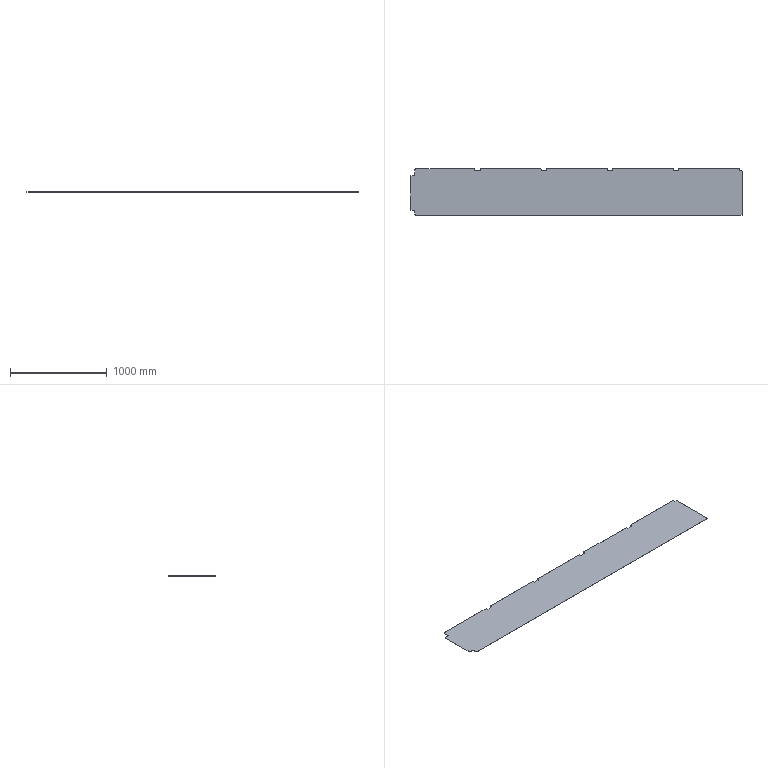Part | SolidWorks | features Fillet 2, ICE 2, Cut 1, FlatPattern 1, SMBaseFlange 1, SheetMetal 1 | 1 solid | 53 faces | box 3434 x 480 x 1.2 mm | volume 1964220 mm3 | plane 28 | cylinder 25 | commonest cylinder face diameters 6 x19 20 x6